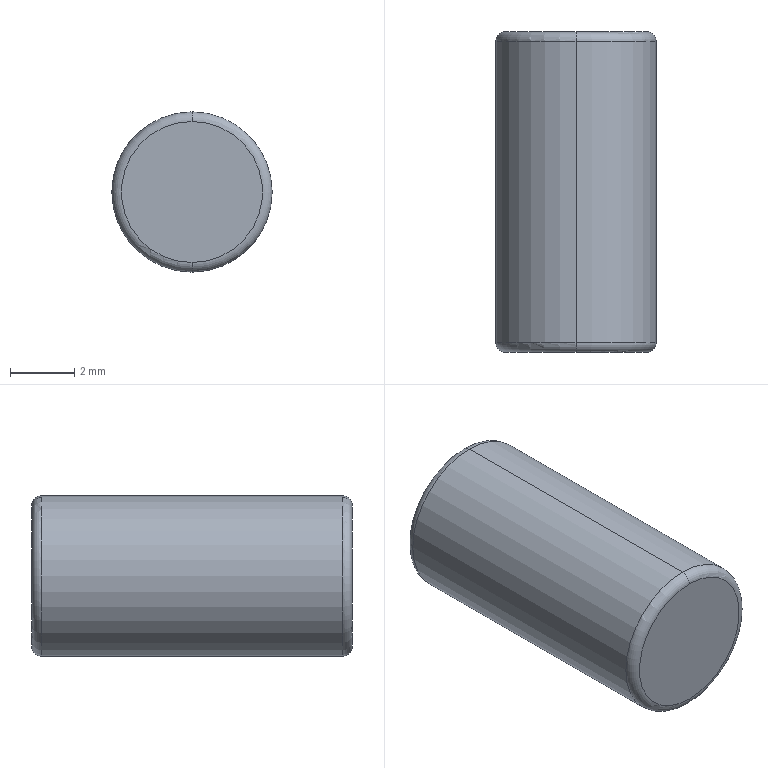Part | STEP file | 5x10 | 1 solid | 8 faces | box 5 x 10 x 5 mm | volume 195.759 mm3 | torus 4 | cylinder 2 | plane 2 | commonest cylinder face diameters 5 x2
STEP:
#1=CARTESIAN_POINT('',(0.,0.,0.));
#2=DIRECTION('',(0.,0.,1.));
#3=DIRECTION('',(1.,0.,0.));
#4=AXIS2_PLACEMENT_3D('',#1,#2,#3);
#5=CARTESIAN_POINT('',(0.,4.7,-2.5));
#6=VERTEX_POINT('',#5);
#7=CARTESIAN_POINT('',(0.,4.7,2.5));
#8=VERTEX_POINT('',#7);
#9=CARTESIAN_POINT('',(0.,4.7,0.));
#10=DIRECTION('',(0.,-1.,0.));
#11=DIRECTION('',(0.,0.,1.));
#12=AXIS2_PLACEMENT_3D('',#9,#10,#11);
#13=CIRCLE('',#12,2.5);
#14=CARTESIAN_POINT('',(0.,4.7,0.));
#15=DIRECTION('',(0.,1.,0.));
#16=DIRECTION('',(0.,0.,1.));
#17=AXIS2_PLACEMENT_3D('',#14,#15,#16);
#18=TOROIDAL_SURFACE('',#17,2.2,0.3);
#19=CARTESIAN_POINT('',(6.283,0.));
#20=DIRECTION('',(-1.,0.));
#21=VECTOR('',#20,1.);
#22=LINE('',#19,#21);
#23=(GEOMETRIC_REPRESENTATION_CONTEXT(2)PARAMETRIC_REPRESENTATION_CONTEXT()REPRESENTATION_CONTEXT('',''));
#24=DEFINITIONAL_REPRESENTATION('',(#22),#23);
#25=PCURVE('',#18,#24);
#26=CARTESIAN_POINT('',(0.,5.,0.));
#27=DIRECTION('',(0.,-1.,0.));
#28=DIRECTION('',(0.,0.,-1.));
#29=AXIS2_PLACEMENT_3D('',#26,#27,#28);
#30=CYLINDRICAL_SURFACE('',#29,2.5);
#31=CARTESIAN_POINT('',(-3.142,0.3));
#32=DIRECTION('',(1.,0.));
#33=VECTOR('',#32,1.);
#34=LINE('',#31,#33);
#35=(GEOMETRIC_REPRESENTATION_CONTEXT(2)PARAMETRIC_REPRESENTATION_CONTEXT()REPRESENTATION_CONTEXT('',''));
#36=DEFINITIONAL_REPRESENTATION('',(#34),#35);
#37=PCURVE('',#30,#36);
#38=SURFACE_CURVE('',#13,(#25,#37),.PCURVE_S1.);
#39=EDGE_CURVE('',#6,#8,#38,.T.);
#40=ORIENTED_EDGE('',*,*,#39,.F.);
#41=CARTESIAN_POINT('',(0.,5.,-2.2));
#42=VERTEX_POINT('',#41);
#43=CARTESIAN_POINT('',(0.,4.7,-2.2));
#44=DIRECTION('',(1.,0.,0.));
#45=DIRECTION('',(0.,0.,-1.));
#46=AXIS2_PLACEMENT_3D('',#43,#44,#45);
#47=CIRCLE('',#46,0.3);
#48=CARTESIAN_POINT('',(3.142,0.));
#49=DIRECTION('',(0.,1.));
#50=VECTOR('',#49,1.);
#51=LINE('',#48,#50);
#52=(GEOMETRIC_REPRESENTATION_CONTEXT(2)PARAMETRIC_REPRESENTATION_CONTEXT()REPRESENTATION_CONTEXT('',''));
#53=DEFINITIONAL_REPRESENTATION('',(#51),#52);
#54=PCURVE('',#18,#53);
#55=CARTESIAN_POINT('',(0.,4.7,0.));
#56=DIRECTION('',(0.,1.,0.));
#57=DIRECTION('',(0.,0.,1.));
#58=AXIS2_PLACEMENT_3D('',#55,#56,#57);
#59=TOROIDAL_SURFACE('',#58,2.2,0.3);
#60=CARTESIAN_POINT('',(3.142,0.));
#61=DIRECTION('',(0.,1.));
#62=VECTOR('',#61,1.);
#63=LINE('',#60,#62);
#64=(GEOMETRIC_REPRESENTATION_CONTEXT(2)PARAMETRIC_REPRESENTATION_CONTEXT()REPRESENTATION_CONTEXT('',''));
#65=DEFINITIONAL_REPRESENTATION('',(#63),#64);
#66=PCURVE('',#59,#65);
#67=SURFACE_CURVE('',#47,(#54,#66),.PCURVE_S1.);
#68=EDGE_CURVE('',#6,#42,#67,.T.);
#69=ORIENTED_EDGE('',*,*,#68,.T.);
#70=CARTESIAN_POINT('',(0.,5.,2.2));
#71=VERTEX_POINT('',#70);
#72=CARTESIAN_POINT('',(0.,5.,0.));
#73=DIRECTION('',(0.,1.,0.));
#74=DIRECTION('',(0.,0.,1.));
#75=AXIS2_PLACEMENT_3D('',#72,#73,#74);
#76=CIRCLE('',#75,2.2);
#77=CARTESIAN_POINT('',(0.,1.571));
#78=DIRECTION('',(1.,0.));
#79=VECTOR('',#78,1.);
#80=LINE('',#77,#79);
#81=(GEOMETRIC_REPRESENTATION_CONTEXT(2)PARAMETRIC_REPRESENTATION_CONTEXT()REPRESENTATION_CONTEXT('',''));
#82=DEFINITIONAL_REPRESENTATION('',(#80),#81);
#83=PCURVE('',#18,#82);
#84=CARTESIAN_POINT('',(0.,5.,0.));
#85=DIRECTION('',(0.,1.,0.));
#86=DIRECTION('',(0.,0.,1.));
#87=AXIS2_PLACEMENT_3D('',#84,#85,#86);
#88=PLANE('',#87);
#89=CARTESIAN_POINT('',(0.,0.));
#90=DIRECTION('',(1.,0.));
#91=AXIS2_PLACEMENT_2D('',#89,#90);
#92=CIRCLE('',#91,2.2);
#93=(GEOMETRIC_REPRESENTATION_CONTEXT(2)PARAMETRIC_REPRESENTATION_CONTEXT()REPRESENTATION_CONTEXT('',''));
#94=DEFINITIONAL_REPRESENTATION('',(#92),#93);
#95=PCURVE('',#88,#94);
#96=SURFACE_CURVE('',#76,(#83,#95),.PCURVE_S1.);
#97=EDGE_CURVE('',#71,#42,#96,.T.);
#98=ORIENTED_EDGE('',*,*,#97,.F.);
#99=CARTESIAN_POINT('',(0.,4.7,2.2));
#100=DIRECTION('',(-1.,0.,0.));
#101=DIRECTION('',(0.,0.,1.));
#102=AXIS2_PLACEMENT_3D('',#99,#100,#101);
#103=CIRCLE('',#102,0.3);
#104=CARTESIAN_POINT('',(0.,0.));
#105=DIRECTION('',(0.,1.));
#106=VECTOR('',#105,1.);
#107=LINE('',#104,#106);
#108=(GEOMETRIC_REPRESENTATION_CONTEXT(2)PARAMETRIC_REPRESENTATION_CONTEXT()REPRESENTATION_CONTEXT('',''));
#109=DEFINITIONAL_REPRESENTATION('',(#107),#108);
#110=PCURVE('',#18,#109);
#111=CARTESIAN_POINT('',(6.283,0.));
#112=DIRECTION('',(0.,1.));
#113=VECTOR('',#112,1.);
#114=LINE('',#111,#113);
#115=(GEOMETRIC_REPRESENTATION_CONTEXT(2)PARAMETRIC_REPRESENTATION_CONTEXT()REPRESENTATION_CONTEXT('',''));
#116=DEFINITIONAL_REPRESENTATION('',(#114),#115);
#117=PCURVE('',#59,#116);
#118=SURFACE_CURVE('',#103,(#110,#117),.PCURVE_S1.);
#119=EDGE_CURVE('',#8,#71,#118,.T.);
#120=ORIENTED_EDGE('',*,*,#119,.F.);
#121=EDGE_LOOP('',(#40,#69,#98,#120));
#122=FACE_BOUND('',#121,.T.);
#123=ADVANCED_FACE('',(#122),#18,.T.);
#124=CARTESIAN_POINT('',(0.,-5.,-2.2));
#125=VERTEX_POINT('',#124);
#126=CARTESIAN_POINT('',(0.,-5.,2.2));
#127=VERTEX_POINT('',#126);
#128=CARTESIAN_POINT('',(0.,-5.,0.));
#129=DIRECTION('',(0.,-1.,0.));
#130=DIRECTION('',(0.,0.,1.));
#131=AXIS2_PLACEMENT_3D('',#128,#129,#130);
#132=CIRCLE('',#131,2.2);
#133=CARTESIAN_POINT('',(0.,-4.7,0.));
#134=DIRECTION('',(0.,1.,0.));
#135=DIRECTION('',(0.,0.,1.));
#136=AXIS2_PLACEMENT_3D('',#133,#134,#135);
#137=TOROIDAL_SURFACE('',#136,2.2,0.3);
#138=CARTESIAN_POINT('',(6.283,4.712));
#139=DIRECTION('',(-1.,0.));
#140=VECTOR('',#139,1.);
#141=LINE('',#138,#140);
#142=(GEOMETRIC_REPRESENTATION_CONTEXT(2)PARAMETRIC_REPRESENTATION_CONTEXT()REPRESENTATION_CONTEXT('',''));
#143=DEFINITIONAL_REPRESENTATION('',(#141),#142);
#144=PCURVE('',#137,#143);
#145=CARTESIAN_POINT('',(0.,-5.,0.));
#146=DIRECTION('',(0.,1.,0.));
#147=DIRECTION('',(0.,0.,1.));
#148=AXIS2_PLACEMENT_3D('',#145,#146,#147);
#149=PLANE('',#148);
#150=CARTESIAN_POINT('',(2.2,0.));
#151=CARTESIAN_POINT('',(2.2,-3.811));
#152=CARTESIAN_POINT('',(-1.1,-1.905));
#153=CARTESIAN_POINT('',(-4.4,0.));
#154=CARTESIAN_POINT('',(-1.1,1.905));
#155=CARTESIAN_POINT('',(2.2,3.811));
#156=CARTESIAN_POINT('',(2.2,0.));
#157=(BOUNDED_CURVE()B_SPLINE_CURVE(2,(#150,#151,#152,#153,#154,#155,#156),.UNSPECIFIED.,.T.,.F.)B_SPLINE_CURVE_WITH_KNOTS((1,2,2,2,2,1),(-2.094,0.,2.094,4.189,6.283,8.378),.UNSPECIFIED.)CURVE()GEOMETRIC_REPRESENTATION_ITEM()RATIONAL_B_SPLINE_CURVE((1.,0.5,1.,0.5,1.,0.5,1.))REPRESENTATION_ITEM(''));
#158=(GEOMETRIC_REPRESENTATION_CONTEXT(2)PARAMETRIC_REPRESENTATION_CONTEXT()REPRESENTATION_CONTEXT('',''));
#159=DEFINITIONAL_REPRESENTATION('',(#157),#158);
#160=PCURVE('',#149,#159);
#161=SURFACE_CURVE('',#132,(#144,#160),.PCURVE_S1.);
#162=EDGE_CURVE('',#125,#127,#161,.T.);
#163=ORIENTED_EDGE('',*,*,#162,.F.);
#164=CARTESIAN_POINT('',(0.,-4.7,-2.5));
#165=VERTEX_POINT('',#164);
#166=CARTESIAN_POINT('',(0.,-4.7,-2.2));
#167=DIRECTION('',(1.,0.,0.));
#168=DIRECTION('',(0.,0.,-1.));
#169=AXIS2_PLACEMENT_3D('',#166,#167,#168);
#170=CIRCLE('',#169,0.3);
#171=CARTESIAN_POINT('',(3.142,0.));
#172=DIRECTION('',(0.,1.));
#173=VECTOR('',#172,1.);
#174=LINE('',#171,#173);
#175=(GEOMETRIC_REPRESENTATION_CONTEXT(2)PARAMETRIC_REPRESENTATION_CONTEXT()REPRESENTATION_CONTEXT('',''));
#176=DEFINITIONAL_REPRESENTATION('',(#174),#175);
#177=PCURVE('',#137,#176);
#178=CARTESIAN_POINT('',(0.,-4.7,0.));
#179=DIRECTION('',(0.,1.,0.));
#180=DIRECTION('',(0.,0.,1.));
#181=AXIS2_PLACEMENT_3D('',#178,#179,#180);
#182=TOROIDAL_SURFACE('',#181,2.2,0.3);
#183=CARTESIAN_POINT('',(3.142,0.));
#184=DIRECTION('',(0.,1.));
#185=VECTOR('',#184,1.);
#186=LINE('',#183,#185);
#187=(GEOMETRIC_REPRESENTATION_CONTEXT(2)PARAMETRIC_REPRESENTATION_CONTEXT()REPRESENTATION_CONTEXT('',''));
#188=DEFINITIONAL_REPRESENTATION('',(#186),#187);
#189=PCURVE('',#182,#188);
#190=SURFACE_CURVE('',#170,(#177,#189),.PCURVE_S1.);
#191=EDGE_CURVE('',#125,#165,#190,.T.);
#192=ORIENTED_EDGE('',*,*,#191,.T.);
#193=CARTESIAN_POINT('',(0.,-4.7,2.5));
#194=VERTEX_POINT('',#193);
#195=CARTESIAN_POINT('',(0.,-4.7,0.));
#196=DIRECTION('',(0.,1.,0.));
#197=DIRECTION('',(0.,0.,1.));
#198=AXIS2_PLACEMENT_3D('',#195,#196,#197);
#199=CIRCLE('',#198,2.5);
#200=CARTESIAN_POINT('',(0.,6.283));
#201=DIRECTION('',(1.,0.));
#202=VECTOR('',#201,1.);
#203=LINE('',#200,#202);
#204=(GEOMETRIC_REPRESENTATION_CONTEXT(2)PARAMETRIC_REPRESENTATION_CONTEXT()REPRESENTATION_CONTEXT('',''));
#205=DEFINITIONAL_REPRESENTATION('',(#203),#204);
#206=PCURVE('',#137,#205);
#207=CARTESIAN_POINT('',(3.142,9.7));
#208=DIRECTION('',(-1.,0.));
#209=VECTOR('',#208,1.);
#210=LINE('',#207,#209);
#211=(GEOMETRIC_REPRESENTATION_CONTEXT(2)PARAMETRIC_REPRESENTATION_CONTEXT()REPRESENTATION_CONTEXT('',''));
#212=DEFINITIONAL_REPRESENTATION('',(#210),#211);
#213=PCURVE('',#30,#212);
#214=SURFACE_CURVE('',#199,(#206,#213),.PCURVE_S1.);
#215=EDGE_CURVE('',#194,#165,#214,.T.);
#216=ORIENTED_EDGE('',*,*,#215,.F.);
#217=CARTESIAN_POINT('',(0.,-4.7,2.2));
#218=DIRECTION('',(-1.,0.,0.));
#219=DIRECTION('',(0.,0.,1.));
#220=AXIS2_PLACEMENT_3D('',#217,#218,#219);
#221=CIRCLE('',#220,0.3);
#222=CARTESIAN_POINT('',(0.,0.));
#223=DIRECTION('',(0.,1.));
#224=VECTOR('',#223,1.);
#225=LINE('',#222,#224);
#226=(GEOMETRIC_REPRESENTATION_CONTEXT(2)PARAMETRIC_REPRESENTATION_CONTEXT()REPRESENTATION_CONTEXT('',''));
#227=DEFINITIONAL_REPRESENTATION('',(#225),#226);
#228=PCURVE('',#137,#227);
#229=CARTESIAN_POINT('',(6.283,0.));
#230=DIRECTION('',(0.,1.));
#231=VECTOR('',#230,1.);
#232=LINE('',#229,#231);
#233=(GEOMETRIC_REPRESENTATION_CONTEXT(2)PARAMETRIC_REPRESENTATION_CONTEXT()REPRESENTATION_CONTEXT('',''));
#234=DEFINITIONAL_REPRESENTATION('',(#232),#233);
#235=PCURVE('',#182,#234);
#236=SURFACE_CURVE('',#221,(#228,#235),.PCURVE_S1.);
#237=EDGE_CURVE('',#127,#194,#236,.T.);
#238=ORIENTED_EDGE('',*,*,#237,.F.);
#239=EDGE_LOOP('',(#163,#192,#216,#238));
#240=FACE_BOUND('',#239,.T.);
#241=ADVANCED_FACE('',(#240),#137,.T.);
#242=ORIENTED_EDGE('',*,*,#39,.T.);
#243=CARTESIAN_POINT('',(0.,5.,2.5));
#244=DIRECTION('',(0.,-1.,0.));
#245=VECTOR('',#244,1.);
#246=LINE('',#243,#245);
#247=CARTESIAN_POINT('',(3.142,0.));
#248=DIRECTION('',(0.,1.));
#249=VECTOR('',#248,1.);
#250=LINE('',#247,#249);
#251=(GEOMETRIC_REPRESENTATION_CONTEXT(2)PARAMETRIC_REPRESENTATION_CONTEXT()REPRESENTATION_CONTEXT('',''));
#252=DEFINITIONAL_REPRESENTATION('',(#250),#251);
#253=PCURVE('',#30,#252);
#254=CARTESIAN_POINT('',(0.,5.,0.));
#255=DIRECTION('',(0.,-1.,0.));
#256=DIRECTION('',(0.,0.,-1.));
#257=AXIS2_PLACEMENT_3D('',#254,#255,#256);
#258=CYLINDRICAL_SURFACE('',#257,2.5);
#259=CARTESIAN_POINT('',(3.142,0.));
#260=DIRECTION('',(0.,1.));
#261=VECTOR('',#260,1.);
#262=LINE('',#259,#261);
#263=(GEOMETRIC_REPRESENTATION_CONTEXT(2)PARAMETRIC_REPRESENTATION_CONTEXT()REPRESENTATION_CONTEXT('',''));
#264=DEFINITIONAL_REPRESENTATION('',(#262),#263);
#265=PCURVE('',#258,#264);
#266=SURFACE_CURVE('',#246,(#253,#265),.PCURVE_S1.);
#267=EDGE_CURVE('',#8,#194,#266,.T.);
#268=ORIENTED_EDGE('',*,*,#267,.T.);
#269=ORIENTED_EDGE('',*,*,#215,.T.);
#270=CARTESIAN_POINT('',(0.,5.,-2.5));
#271=DIRECTION('',(0.,-1.,0.));
#272=VECTOR('',#271,1.);
#273=LINE('',#270,#272);
#274=CARTESIAN_POINT('',(0.,0.));
#275=DIRECTION('',(0.,1.));
#276=VECTOR('',#275,1.);
#277=LINE('',#274,#276);
#278=(GEOMETRIC_REPRESENTATION_CONTEXT(2)PARAMETRIC_REPRESENTATION_CONTEXT()REPRESENTATION_CONTEXT('',''));
#279=DEFINITIONAL_REPRESENTATION('',(#277),#278);
#280=PCURVE('',#30,#279);
#281=CARTESIAN_POINT('',(6.283,0.));
#282=DIRECTION('',(0.,1.));
#283=VECTOR('',#282,1.);
#284=LINE('',#281,#283);
#285=(GEOMETRIC_REPRESENTATION_CONTEXT(2)PARAMETRIC_REPRESENTATION_CONTEXT()REPRESENTATION_CONTEXT('',''));
#286=DEFINITIONAL_REPRESENTATION('',(#284),#285);
#287=PCURVE('',#258,#286);
#288=SURFACE_CURVE('',#273,(#280,#287),.PCURVE_S1.);
#289=EDGE_CURVE('',#6,#165,#288,.T.);
#290=ORIENTED_EDGE('',*,*,#289,.F.);
#291=EDGE_LOOP('',(#242,#268,#269,#290));
#292=FACE_BOUND('',#291,.T.);
#293=ADVANCED_FACE('',(#292),#30,.T.);
#294=ORIENTED_EDGE('',*,*,#267,.F.);
#295=CARTESIAN_POINT('',(0.,4.7,0.));
#296=DIRECTION('',(0.,-1.,0.));
#297=DIRECTION('',(0.,0.,1.));
#298=AXIS2_PLACEMENT_3D('',#295,#296,#297);
#299=CIRCLE('',#298,2.5);
#300=CARTESIAN_POINT('',(3.142,0.3));
#301=DIRECTION('',(1.,0.));
#302=VECTOR('',#301,1.);
#303=LINE('',#300,#302);
#304=(GEOMETRIC_REPRESENTATION_CONTEXT(2)PARAMETRIC_REPRESENTATION_CONTEXT()REPRESENTATION_CONTEXT('',''));
#305=DEFINITIONAL_REPRESENTATION('',(#303),#304);
#306=PCURVE('',#258,#305);
#307=CARTESIAN_POINT('',(6.283,0.));
#308=DIRECTION('',(-1.,0.));
#309=VECTOR('',#308,1.);
#310=LINE('',#307,#309);
#311=(GEOMETRIC_REPRESENTATION_CONTEXT(2)PARAMETRIC_REPRESENTATION_CONTEXT()REPRESENTATION_CONTEXT('',''));
#312=DEFINITIONAL_REPRESENTATION('',(#310),#311);
#313=PCURVE('',#59,#312);
#314=SURFACE_CURVE('',#299,(#306,#313),.PCURVE_S1.);
#315=EDGE_CURVE('',#8,#6,#314,.T.);
#316=ORIENTED_EDGE('',*,*,#315,.T.);
#317=ORIENTED_EDGE('',*,*,#289,.T.);
#318=CARTESIAN_POINT('',(0.,-4.7,0.));
#319=DIRECTION('',(0.,1.,0.));
#320=DIRECTION('',(0.,0.,1.));
#321=AXIS2_PLACEMENT_3D('',#318,#319,#320);
#322=CIRCLE('',#321,2.5);
#323=CARTESIAN_POINT('',(9.425,9.7));
#324=DIRECTION('',(-1.,0.));
#325=VECTOR('',#324,1.);
#326=LINE('',#323,#325);
#327=(GEOMETRIC_REPRESENTATION_CONTEXT(2)PARAMETRIC_REPRESENTATION_CONTEXT()REPRESENTATION_CONTEXT('',''));
#328=DEFINITIONAL_REPRESENTATION('',(#326),#327);
#329=PCURVE('',#258,#328);
#330=CARTESIAN_POINT('',(0.,6.283));
#331=DIRECTION('',(1.,0.));
#332=VECTOR('',#331,1.);
#333=LINE('',#330,#332);
#334=(GEOMETRIC_REPRESENTATION_CONTEXT(2)PARAMETRIC_REPRESENTATION_CONTEXT()REPRESENTATION_CONTEXT('',''));
#335=DEFINITIONAL_REPRESENTATION('',(#333),#334);
#336=PCURVE('',#182,#335);
#337=SURFACE_CURVE('',#322,(#329,#336),.PCURVE_S1.);
#338=EDGE_CURVE('',#165,#194,#337,.T.);
#339=ORIENTED_EDGE('',*,*,#338,.T.);
#340=EDGE_LOOP('',(#294,#316,#317,#339));
#341=FACE_BOUND('',#340,.T.);
#342=ADVANCED_FACE('',(#341),#258,.T.);
#343=ORIENTED_EDGE('',*,*,#97,.T.);
#344=CARTESIAN_POINT('',(0.,5.,0.));
#345=DIRECTION('',(0.,1.,0.));
#346=DIRECTION('',(0.,0.,1.));
#347=AXIS2_PLACEMENT_3D('',#344,#345,#346);
#348=CIRCLE('',#347,2.2);
#349=CARTESIAN_POINT('',(0.,0.));
#350=DIRECTION('',(1.,0.));
#351=AXIS2_PLACEMENT_2D('',#349,#350);
#352=CIRCLE('',#351,2.2);
#353=(GEOMETRIC_REPRESENTATION_CONTEXT(2)PARAMETRIC_REPRESENTATION_CONTEXT()REPRESENTATION_CONTEXT('',''));
#354=DEFINITIONAL_REPRESENTATION('',(#352),#353);
#355=PCURVE('',#88,#354);
#356=CARTESIAN_POINT('',(0.,1.571));
#357=DIRECTION('',(1.,0.));
#358=VECTOR('',#357,1.);
#359=LINE('',#356,#358);
#360=(GEOMETRIC_REPRESENTATION_CONTEXT(2)PARAMETRIC_REPRESENTATION_CONTEXT()REPRESENTATION_CONTEXT('',''));
#361=DEFINITIONAL_REPRESENTATION('',(#359),#360);
#362=PCURVE('',#59,#361);
#363=SURFACE_CURVE('',#348,(#355,#362),.PCURVE_S1.);
#364=EDGE_CURVE('',#42,#71,#363,.T.);
#365=ORIENTED_EDGE('',*,*,#364,.T.);
#366=EDGE_LOOP('',(#343,#365));
#367=FACE_BOUND('',#366,.T.);
#368=ADVANCED_FACE('',(#367),#88,.T.);
#369=CARTESIAN_POINT('',(0.,-5.,0.));
#370=DIRECTION('',(0.,-1.,0.));
#371=DIRECTION('',(0.,0.,1.));
#372=AXIS2_PLACEMENT_3D('',#369,#370,#371);
#373=CIRCLE('',#372,2.2);
#374=CARTESIAN_POINT('',(2.2,0.));
#375=CARTESIAN_POINT('',(2.2,-3.811));
#376=CARTESIAN_POINT('',(-1.1,-1.905));
#377=CARTESIAN_POINT('',(-4.4,0.));
#378=CARTESIAN_POINT('',(-1.1,1.905));
#379=CARTESIAN_POINT('',(2.2,3.811));
#380=CARTESIAN_POINT('',(2.2,0.));
#381=(BOUNDED_CURVE()B_SPLINE_CURVE(2,(#374,#375,#376,#377,#378,#379,#380),.UNSPECIFIED.,.T.,.F.)B_SPLINE_CURVE_WITH_KNOTS((1,2,2,2,2,1),(-2.094,0.,2.094,4.189,6.283,8.378),.UNSPECIFIED.)CURVE()GEOMETRIC_REPRESENTATION_ITEM()RATIONAL_B_SPLINE_CURVE((1.,0.5,1.,0.5,1.,0.5,1.))REPRESENTATION_ITEM(''));
#382=(GEOMETRIC_REPRESENTATION_CONTEXT(2)PARAMETRIC_REPRESENTATION_CONTEXT()REPRESENTATION_CONTEXT('',''));
#383=DEFINITIONAL_REPRESENTATION('',(#381),#382);
#384=PCURVE('',#149,#383);
#385=CARTESIAN_POINT('',(6.283,4.712));
#386=DIRECTION('',(-1.,0.));
#387=VECTOR('',#386,1.);
#388=LINE('',#385,#387);
#389=(GEOMETRIC_REPRESENTATION_CONTEXT(2)PARAMETRIC_REPRESENTATION_CONTEXT()REPRESENTATION_CONTEXT('',''));
#390=DEFINITIONAL_REPRESENTATION('',(#388),#389);
#391=PCURVE('',#182,#390);
#392=SURFACE_CURVE('',#373,(#384,#391),.PCURVE_S1.);
#393=EDGE_CURVE('',#127,#125,#392,.T.);
#394=ORIENTED_EDGE('',*,*,#393,.T.);
#395=ORIENTED_EDGE('',*,*,#162,.T.);
#396=EDGE_LOOP('',(#394,#395));
#397=FACE_BOUND('',#396,.T.);
#398=ADVANCED_FACE('',(#397),#149,.F.);
#399=ORIENTED_EDGE('',*,*,#191,.F.);
#400=ORIENTED_EDGE('',*,*,#393,.F.);
#401=ORIENTED_EDGE('',*,*,#237,.T.);
#402=ORIENTED_EDGE('',*,*,#338,.F.);
#403=EDGE_LOOP('',(#399,#400,#401,#402));
#404=FACE_BOUND('',#403,.T.);
#405=ADVANCED_FACE('',(#404),#182,.T.);
#406=ORIENTED_EDGE('',*,*,#68,.F.);
#407=ORIENTED_EDGE('',*,*,#315,.F.);
#408=ORIENTED_EDGE('',*,*,#119,.T.);
#409=ORIENTED_EDGE('',*,*,#364,.F.);
#410=EDGE_LOOP('',(#406,#407,#408,#409));
#411=FACE_BOUND('',#410,.T.);
#412=ADVANCED_FACE('',(#411),#59,.T.);
#413=CLOSED_SHELL('',(#123,#241,#293,#342,#368,#398,#405,#412));
#414=MANIFOLD_SOLID_BREP('',#413);
#415=(LENGTH_UNIT()NAMED_UNIT(*)SI_UNIT(.MILLI.,.METRE.));
#416=UNCERTAINTY_MEASURE_WITH_UNIT(LENGTH_MEASURE(0.0000001),#415,'','');
#417=(NAMED_UNIT(*)PLANE_ANGLE_UNIT()SI_UNIT($,.RADIAN.));
#418=(NAMED_UNIT(*)SI_UNIT($,.STERADIAN.)SOLID_ANGLE_UNIT());
#419=(GEOMETRIC_REPRESENTATION_CONTEXT(3)GLOBAL_UNCERTAINTY_ASSIGNED_CONTEXT((#416))GLOBAL_UNIT_ASSIGNED_CONTEXT((#415,#417,#418))REPRESENTATION_CONTEXT('',''));
#420=ADVANCED_BREP_SHAPE_REPRESENTATION('',(#4,#414),#419);